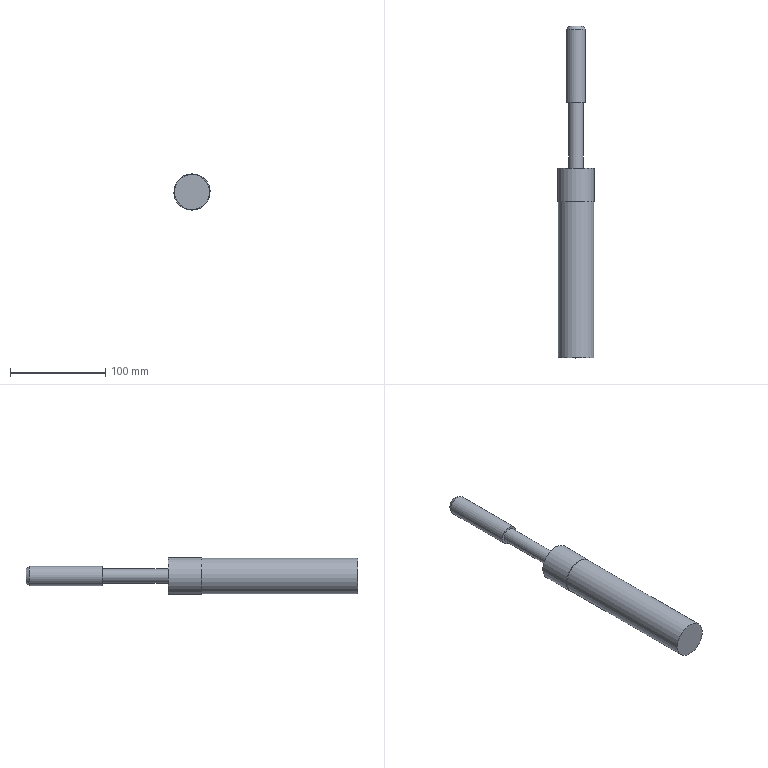Part | STEP file | TOCHA_DE_SOLDA_TBI | 1 solid | 10 faces | box 38 x 348 x 38 mm | volume 253151 mm3 | plane 5 | cylinder 4 | cone 1 | commonest cylinder face diameters 15 x1 20 x1 37 x1 38 x1
STEP:
#1=CARTESIAN_POINT('',(0.,0.,0.));
#2=DIRECTION('',(0.,0.,1.));
#3=DIRECTION('',(1.,0.,0.));
#4=AXIS2_PLACEMENT_3D('',#1,#2,#3);
#5=CARTESIAN_POINT('',(-3.596,-90.,-6.582));
#6=VERTEX_POINT('',#5);
#7=CARTESIAN_POINT('',(0.,-90.,0.));
#8=DIRECTION('',(0.,1.,0.));
#9=DIRECTION('',(1.,0.,0.));
#10=AXIS2_PLACEMENT_3D('',#7,#8,#9);
#11=CIRCLE('',#10,7.5);
#12=CARTESIAN_POINT('',(0.,-184.,0.));
#13=DIRECTION('',(0.,1.,0.));
#14=DIRECTION('',(0.4794,0.,0.8776));
#15=AXIS2_PLACEMENT_3D('',#12,#13,#14);
#16=CYLINDRICAL_SURFACE('',#15,7.5);
#17=CARTESIAN_POINT('',(1.071,94.));
#18=DIRECTION('',(1.,0.));
#19=VECTOR('',#18,1.);
#20=LINE('',#17,#19);
#21=(GEOMETRIC_REPRESENTATION_CONTEXT(2)PARAMETRIC_REPRESENTATION_CONTEXT()REPRESENTATION_CONTEXT('',''));
#22=DEFINITIONAL_REPRESENTATION('',(#20),#21);
#23=PCURVE('',#16,#22);
#24=CARTESIAN_POINT('',(0.,-90.,10.));
#25=DIRECTION('',(0.,1.,0.));
#26=DIRECTION('',(0.,0.,1.));
#27=AXIS2_PLACEMENT_3D('',#24,#25,#26);
#28=PLANE('',#27);
#29=CARTESIAN_POINT('',(-10.,0.));
#30=DIRECTION('',(0.,1.));
#31=AXIS2_PLACEMENT_2D('',#29,#30);
#32=CIRCLE('',#31,7.5);
#33=(GEOMETRIC_REPRESENTATION_CONTEXT(2)PARAMETRIC_REPRESENTATION_CONTEXT()REPRESENTATION_CONTEXT('',''));
#34=DEFINITIONAL_REPRESENTATION('',(#32),#33);
#35=PCURVE('',#28,#34);
#36=SURFACE_CURVE('',#11,(#23,#35),.PCURVE_S1.);
#37=EDGE_CURVE('',#6,#6,#36,.T.);
#38=ORIENTED_EDGE('',*,*,#37,.F.);
#39=CARTESIAN_POINT('',(-3.596,-159.,-6.582));
#40=VERTEX_POINT('',#39);
#41=CARTESIAN_POINT('',(-3.596,-159.,-6.582));
#42=CARTESIAN_POINT('',(-3.596,-90.,-6.582));
#43=B_SPLINE_CURVE_WITH_KNOTS('',1,(#41,#42),.UNSPECIFIED.,.F.,.F.,(2,2),(25.,94.),.PIECEWISE_BEZIER_KNOTS.);
#44=CARTESIAN_POINT('',(3.142,0.));
#45=DIRECTION('',(0.,1.));
#46=VECTOR('',#45,1.);
#47=LINE('',#44,#46);
#48=(GEOMETRIC_REPRESENTATION_CONTEXT(2)PARAMETRIC_REPRESENTATION_CONTEXT()REPRESENTATION_CONTEXT('',''));
#49=DEFINITIONAL_REPRESENTATION('',(#47),#48);
#50=PCURVE('',#16,#49);
#51=CARTESIAN_POINT('',(9.425,0.));
#52=DIRECTION('',(0.,1.));
#53=VECTOR('',#52,1.);
#54=LINE('',#51,#53);
#55=(GEOMETRIC_REPRESENTATION_CONTEXT(2)PARAMETRIC_REPRESENTATION_CONTEXT()REPRESENTATION_CONTEXT('',''));
#56=DEFINITIONAL_REPRESENTATION('',(#54),#55);
#57=PCURVE('',#16,#56);
#58=SEAM_CURVE('',#43,(#50,#57),.PCURVE_S1.);
#59=EDGE_CURVE('',#40,#6,#58,.T.);
#60=ORIENTED_EDGE('',*,*,#59,.F.);
#61=CARTESIAN_POINT('',(0.,-159.,0.));
#62=DIRECTION('',(0.,1.,0.));
#63=DIRECTION('',(1.,0.,0.));
#64=AXIS2_PLACEMENT_3D('',#61,#62,#63);
#65=CIRCLE('',#64,7.5);
#66=CARTESIAN_POINT('',(1.071,25.));
#67=DIRECTION('',(1.,0.));
#68=VECTOR('',#67,1.);
#69=LINE('',#66,#68);
#70=(GEOMETRIC_REPRESENTATION_CONTEXT(2)PARAMETRIC_REPRESENTATION_CONTEXT()REPRESENTATION_CONTEXT('',''));
#71=DEFINITIONAL_REPRESENTATION('',(#69),#70);
#72=PCURVE('',#16,#71);
#73=CARTESIAN_POINT('',(0.,-159.,7.5));
#74=DIRECTION('',(0.,1.,0.));
#75=DIRECTION('',(0.,0.,1.));
#76=AXIS2_PLACEMENT_3D('',#73,#74,#75);
#77=PLANE('',#76);
#78=CARTESIAN_POINT('',(-7.5,0.));
#79=DIRECTION('',(0.,1.));
#80=AXIS2_PLACEMENT_2D('',#78,#79);
#81=CIRCLE('',#80,7.5);
#82=(GEOMETRIC_REPRESENTATION_CONTEXT(2)PARAMETRIC_REPRESENTATION_CONTEXT()REPRESENTATION_CONTEXT('',''));
#83=DEFINITIONAL_REPRESENTATION('',(#81),#82);
#84=PCURVE('',#77,#83);
#85=SURFACE_CURVE('',#65,(#72,#84),.PCURVE_S1.);
#86=EDGE_CURVE('',#40,#40,#85,.T.);
#87=ORIENTED_EDGE('',*,*,#86,.T.);
#88=ORIENTED_EDGE('',*,*,#59,.T.);
#89=EDGE_LOOP('',(#38,#60,#87,#88));
#90=FACE_BOUND('',#89,.T.);
#91=ADVANCED_FACE('',(#90),#16,.T.);
#92=CARTESIAN_POINT('',(-9.109,-159.,-16.674));
#93=VERTEX_POINT('',#92);
#94=CARTESIAN_POINT('',(0.,-159.,0.));
#95=DIRECTION('',(0.,1.,0.));
#96=DIRECTION('',(1.,0.,0.));
#97=AXIS2_PLACEMENT_3D('',#94,#95,#96);
#98=CIRCLE('',#97,19.);
#99=CARTESIAN_POINT('',(0.,-184.,0.));
#100=DIRECTION('',(0.,1.,0.));
#101=DIRECTION('',(0.4794,0.,0.8776));
#102=AXIS2_PLACEMENT_3D('',#99,#100,#101);
#103=CYLINDRICAL_SURFACE('',#102,19.);
#104=CARTESIAN_POINT('',(1.071,25.));
#105=DIRECTION('',(1.,0.));
#106=VECTOR('',#105,1.);
#107=LINE('',#104,#106);
#108=(GEOMETRIC_REPRESENTATION_CONTEXT(2)PARAMETRIC_REPRESENTATION_CONTEXT()REPRESENTATION_CONTEXT('',''));
#109=DEFINITIONAL_REPRESENTATION('',(#107),#108);
#110=PCURVE('',#103,#109);
#111=CARTESIAN_POINT('',(-7.5,0.));
#112=DIRECTION('',(0.,1.));
#113=AXIS2_PLACEMENT_2D('',#111,#112);
#114=CIRCLE('',#113,19.);
#115=(GEOMETRIC_REPRESENTATION_CONTEXT(2)PARAMETRIC_REPRESENTATION_CONTEXT()REPRESENTATION_CONTEXT('',''));
#116=DEFINITIONAL_REPRESENTATION('',(#114),#115);
#117=PCURVE('',#77,#116);
#118=SURFACE_CURVE('',#98,(#110,#117),.PCURVE_S1.);
#119=EDGE_CURVE('',#93,#93,#118,.T.);
#120=ORIENTED_EDGE('',*,*,#119,.F.);
#121=CARTESIAN_POINT('',(-9.109,-194.,-16.674));
#122=VERTEX_POINT('',#121);
#123=CARTESIAN_POINT('',(-9.109,-194.,-16.674));
#124=CARTESIAN_POINT('',(-9.109,-159.,-16.674));
#125=B_SPLINE_CURVE_WITH_KNOTS('',1,(#123,#124),.UNSPECIFIED.,.F.,.F.,(2,2),(-10.,25.),.PIECEWISE_BEZIER_KNOTS.);
#126=CARTESIAN_POINT('',(3.142,0.));
#127=DIRECTION('',(0.,1.));
#128=VECTOR('',#127,1.);
#129=LINE('',#126,#128);
#130=(GEOMETRIC_REPRESENTATION_CONTEXT(2)PARAMETRIC_REPRESENTATION_CONTEXT()REPRESENTATION_CONTEXT('',''));
#131=DEFINITIONAL_REPRESENTATION('',(#129),#130);
#132=PCURVE('',#103,#131);
#133=CARTESIAN_POINT('',(9.425,0.));
#134=DIRECTION('',(0.,1.));
#135=VECTOR('',#134,1.);
#136=LINE('',#133,#135);
#137=(GEOMETRIC_REPRESENTATION_CONTEXT(2)PARAMETRIC_REPRESENTATION_CONTEXT()REPRESENTATION_CONTEXT('',''));
#138=DEFINITIONAL_REPRESENTATION('',(#136),#137);
#139=PCURVE('',#103,#138);
#140=SEAM_CURVE('',#125,(#132,#139),.PCURVE_S1.);
#141=EDGE_CURVE('',#122,#93,#140,.T.);
#142=ORIENTED_EDGE('',*,*,#141,.F.);
#143=CARTESIAN_POINT('',(0.,-194.,0.));
#144=DIRECTION('',(0.,1.,0.));
#145=DIRECTION('',(1.,0.,0.));
#146=AXIS2_PLACEMENT_3D('',#143,#144,#145);
#147=CIRCLE('',#146,19.);
#148=CARTESIAN_POINT('',(1.071,-10.));
#149=DIRECTION('',(1.,0.));
#150=VECTOR('',#149,1.);
#151=LINE('',#148,#150);
#152=(GEOMETRIC_REPRESENTATION_CONTEXT(2)PARAMETRIC_REPRESENTATION_CONTEXT()REPRESENTATION_CONTEXT('',''));
#153=DEFINITIONAL_REPRESENTATION('',(#151),#152);
#154=PCURVE('',#103,#153);
#155=CARTESIAN_POINT('',(0.,-194.,19.));
#156=DIRECTION('',(0.,1.,0.));
#157=DIRECTION('',(0.,0.,1.));
#158=AXIS2_PLACEMENT_3D('',#155,#156,#157);
#159=PLANE('',#158);
#160=CARTESIAN_POINT('',(-19.,0.));
#161=DIRECTION('',(0.,1.));
#162=AXIS2_PLACEMENT_2D('',#160,#161);
#163=CIRCLE('',#162,19.);
#164=(GEOMETRIC_REPRESENTATION_CONTEXT(2)PARAMETRIC_REPRESENTATION_CONTEXT()REPRESENTATION_CONTEXT('',''));
#165=DEFINITIONAL_REPRESENTATION('',(#163),#164);
#166=PCURVE('',#159,#165);
#167=SURFACE_CURVE('',#147,(#154,#166),.PCURVE_S1.);
#168=EDGE_CURVE('',#122,#122,#167,.T.);
#169=ORIENTED_EDGE('',*,*,#168,.T.);
#170=ORIENTED_EDGE('',*,*,#141,.T.);
#171=EDGE_LOOP('',(#120,#142,#169,#170));
#172=FACE_BOUND('',#171,.T.);
#173=ADVANCED_FACE('',(#172),#103,.T.);
#174=CARTESIAN_POINT('',(-8.869,-194.,-16.235));
#175=VERTEX_POINT('',#174);
#176=CARTESIAN_POINT('',(0.,-194.,0.));
#177=DIRECTION('',(0.,1.,0.));
#178=DIRECTION('',(1.,0.,0.));
#179=AXIS2_PLACEMENT_3D('',#176,#177,#178);
#180=CIRCLE('',#179,18.5);
#181=CARTESIAN_POINT('',(0.,-184.,0.));
#182=DIRECTION('',(0.,1.,0.));
#183=DIRECTION('',(0.4794,0.,0.8776));
#184=AXIS2_PLACEMENT_3D('',#181,#182,#183);
#185=CYLINDRICAL_SURFACE('',#184,18.5);
#186=CARTESIAN_POINT('',(1.071,-10.));
#187=DIRECTION('',(1.,0.));
#188=VECTOR('',#187,1.);
#189=LINE('',#186,#188);
#190=(GEOMETRIC_REPRESENTATION_CONTEXT(2)PARAMETRIC_REPRESENTATION_CONTEXT()REPRESENTATION_CONTEXT('',''));
#191=DEFINITIONAL_REPRESENTATION('',(#189),#190);
#192=PCURVE('',#185,#191);
#193=CARTESIAN_POINT('',(-19.,0.));
#194=DIRECTION('',(0.,1.));
#195=AXIS2_PLACEMENT_2D('',#193,#194);
#196=CIRCLE('',#195,18.5);
#197=(GEOMETRIC_REPRESENTATION_CONTEXT(2)PARAMETRIC_REPRESENTATION_CONTEXT()REPRESENTATION_CONTEXT('',''));
#198=DEFINITIONAL_REPRESENTATION('',(#196),#197);
#199=PCURVE('',#159,#198);
#200=SURFACE_CURVE('',#180,(#192,#199),.PCURVE_S1.);
#201=EDGE_CURVE('',#175,#175,#200,.T.);
#202=ORIENTED_EDGE('',*,*,#201,.F.);
#203=CARTESIAN_POINT('',(-8.869,-358.,-16.235));
#204=VERTEX_POINT('',#203);
#205=CARTESIAN_POINT('',(-8.869,-358.,-16.235));
#206=CARTESIAN_POINT('',(-8.869,-194.,-16.235));
#207=B_SPLINE_CURVE_WITH_KNOTS('',1,(#205,#206),.UNSPECIFIED.,.F.,.F.,(2,2),(-174.,-10.),.PIECEWISE_BEZIER_KNOTS.);
#208=CARTESIAN_POINT('',(3.142,0.));
#209=DIRECTION('',(0.,1.));
#210=VECTOR('',#209,1.);
#211=LINE('',#208,#210);
#212=(GEOMETRIC_REPRESENTATION_CONTEXT(2)PARAMETRIC_REPRESENTATION_CONTEXT()REPRESENTATION_CONTEXT('',''));
#213=DEFINITIONAL_REPRESENTATION('',(#211),#212);
#214=PCURVE('',#185,#213);
#215=CARTESIAN_POINT('',(9.425,0.));
#216=DIRECTION('',(0.,1.));
#217=VECTOR('',#216,1.);
#218=LINE('',#215,#217);
#219=(GEOMETRIC_REPRESENTATION_CONTEXT(2)PARAMETRIC_REPRESENTATION_CONTEXT()REPRESENTATION_CONTEXT('',''));
#220=DEFINITIONAL_REPRESENTATION('',(#218),#219);
#221=PCURVE('',#185,#220);
#222=SEAM_CURVE('',#207,(#214,#221),.PCURVE_S1.);
#223=EDGE_CURVE('',#204,#175,#222,.T.);
#224=ORIENTED_EDGE('',*,*,#223,.F.);
#225=CARTESIAN_POINT('',(0.,-358.,0.));
#226=DIRECTION('',(0.,1.,0.));
#227=DIRECTION('',(1.,0.,0.));
#228=AXIS2_PLACEMENT_3D('',#225,#226,#227);
#229=CIRCLE('',#228,18.5);
#230=CARTESIAN_POINT('',(1.071,-174.));
#231=DIRECTION('',(1.,0.));
#232=VECTOR('',#231,1.);
#233=LINE('',#230,#232);
#234=(GEOMETRIC_REPRESENTATION_CONTEXT(2)PARAMETRIC_REPRESENTATION_CONTEXT()REPRESENTATION_CONTEXT('',''));
#235=DEFINITIONAL_REPRESENTATION('',(#233),#234);
#236=PCURVE('',#185,#235);
#237=CARTESIAN_POINT('',(0.,-358.,18.5));
#238=DIRECTION('',(0.,1.,0.));
#239=DIRECTION('',(0.,0.,1.));
#240=AXIS2_PLACEMENT_3D('',#237,#238,#239);
#241=PLANE('',#240);
#242=CARTESIAN_POINT('',(-18.5,0.));
#243=DIRECTION('',(0.,1.));
#244=AXIS2_PLACEMENT_2D('',#242,#243);
#245=CIRCLE('',#244,18.5);
#246=(GEOMETRIC_REPRESENTATION_CONTEXT(2)PARAMETRIC_REPRESENTATION_CONTEXT()REPRESENTATION_CONTEXT('',''));
#247=DEFINITIONAL_REPRESENTATION('',(#245),#246);
#248=PCURVE('',#241,#247);
#249=SURFACE_CURVE('',#229,(#236,#248),.PCURVE_S1.);
#250=EDGE_CURVE('',#204,#204,#249,.T.);
#251=ORIENTED_EDGE('',*,*,#250,.T.);
#252=ORIENTED_EDGE('',*,*,#223,.T.);
#253=EDGE_LOOP('',(#202,#224,#251,#252));
#254=FACE_BOUND('',#253,.T.);
#255=ADVANCED_FACE('',(#254),#185,.T.);
#256=CARTESIAN_POINT('',(-4.794,-90.,-8.776));
#257=VERTEX_POINT('',#256);
#258=CARTESIAN_POINT('',(0.,-90.,0.));
#259=DIRECTION('',(0.,1.,0.));
#260=DIRECTION('',(1.,0.,0.));
#261=AXIS2_PLACEMENT_3D('',#258,#259,#260);
#262=CIRCLE('',#261,10.);
#263=CARTESIAN_POINT('',(-10.,0.));
#264=DIRECTION('',(0.,1.));
#265=AXIS2_PLACEMENT_2D('',#263,#264);
#266=CIRCLE('',#265,10.);
#267=(GEOMETRIC_REPRESENTATION_CONTEXT(2)PARAMETRIC_REPRESENTATION_CONTEXT()REPRESENTATION_CONTEXT('',''));
#268=DEFINITIONAL_REPRESENTATION('',(#266),#267);
#269=PCURVE('',#28,#268);
#270=CARTESIAN_POINT('',(0.,-184.,0.));
#271=DIRECTION('',(0.,1.,0.));
#272=DIRECTION('',(0.4794,0.,0.8776));
#273=AXIS2_PLACEMENT_3D('',#270,#271,#272);
#274=CYLINDRICAL_SURFACE('',#273,10.);
#275=CARTESIAN_POINT('',(1.071,94.));
#276=DIRECTION('',(1.,0.));
#277=VECTOR('',#276,1.);
#278=LINE('',#275,#277);
#279=(GEOMETRIC_REPRESENTATION_CONTEXT(2)PARAMETRIC_REPRESENTATION_CONTEXT()REPRESENTATION_CONTEXT('',''));
#280=DEFINITIONAL_REPRESENTATION('',(#278),#279);
#281=PCURVE('',#274,#280);
#282=SURFACE_CURVE('',#262,(#269,#281),.PCURVE_S1.);
#283=EDGE_CURVE('',#257,#257,#282,.T.);
#284=ORIENTED_EDGE('',*,*,#283,.F.);
#285=EDGE_LOOP('',(#284));
#286=FACE_BOUND('',#285,.T.);
#287=ORIENTED_EDGE('',*,*,#37,.T.);
#288=EDGE_LOOP('',(#287));
#289=FACE_BOUND('',#288,.T.);
#290=ADVANCED_FACE('',(#286,#289),#28,.F.);
#291=ORIENTED_EDGE('',*,*,#119,.T.);
#292=EDGE_LOOP('',(#291));
#293=FACE_BOUND('',#292,.T.);
#294=ORIENTED_EDGE('',*,*,#86,.F.);
#295=EDGE_LOOP('',(#294));
#296=FACE_BOUND('',#295,.T.);
#297=ADVANCED_FACE('',(#293,#296),#77,.T.);
#298=ORIENTED_EDGE('',*,*,#168,.F.);
#299=EDGE_LOOP('',(#298));
#300=FACE_BOUND('',#299,.T.);
#301=ORIENTED_EDGE('',*,*,#201,.T.);
#302=EDGE_LOOP('',(#301));
#303=FACE_BOUND('',#302,.T.);
#304=ADVANCED_FACE('',(#300,#303),#159,.F.);
#305=ORIENTED_EDGE('',*,*,#250,.F.);
#306=EDGE_LOOP('',(#305));
#307=FACE_BOUND('',#306,.T.);
#308=ADVANCED_FACE('',(#307),#241,.F.);
#309=CARTESIAN_POINT('',(-4.794,-13.464,-8.776));
#310=VERTEX_POINT('',#309);
#311=CARTESIAN_POINT('',(0.,-13.464,0.));
#312=DIRECTION('',(0.,1.,0.));
#313=DIRECTION('',(1.,0.,0.));
#314=AXIS2_PLACEMENT_3D('',#311,#312,#313);
#315=CIRCLE('',#314,10.);
#316=CARTESIAN_POINT('',(1.071,170.536));
#317=DIRECTION('',(1.,0.));
#318=VECTOR('',#317,1.);
#319=LINE('',#316,#318);
#320=(GEOMETRIC_REPRESENTATION_CONTEXT(2)PARAMETRIC_REPRESENTATION_CONTEXT()REPRESENTATION_CONTEXT('',''));
#321=DEFINITIONAL_REPRESENTATION('',(#319),#320);
#322=PCURVE('',#274,#321);
#323=CARTESIAN_POINT('',(0.,2.124,0.));
#324=DIRECTION('',(0.,-1.,0.));
#325=DIRECTION('',(-0.4164,0.,-0.9092));
#326=AXIS2_PLACEMENT_3D('',#323,#324,#325);
#327=CONICAL_SURFACE('',#326,1.,0.5236);
#328=CARTESIAN_POINT('',(14.567,15.588));
#329=DIRECTION('',(-1.,0.));
#330=VECTOR('',#329,1.);
#331=LINE('',#328,#330);
#332=(GEOMETRIC_REPRESENTATION_CONTEXT(2)PARAMETRIC_REPRESENTATION_CONTEXT()REPRESENTATION_CONTEXT('',''));
#333=DEFINITIONAL_REPRESENTATION('',(#331),#332);
#334=PCURVE('',#327,#333);
#335=SURFACE_CURVE('',#315,(#322,#334),.PCURVE_S1.);
#336=EDGE_CURVE('',#310,#310,#335,.T.);
#337=ORIENTED_EDGE('',*,*,#336,.F.);
#338=CARTESIAN_POINT('',(-4.794,-90.,-8.776));
#339=CARTESIAN_POINT('',(-4.794,-13.464,-8.776));
#340=B_SPLINE_CURVE_WITH_KNOTS('',1,(#338,#339),.UNSPECIFIED.,.F.,.F.,(2,2),(94.,170.536),.PIECEWISE_BEZIER_KNOTS.);
#341=CARTESIAN_POINT('',(3.142,0.));
#342=DIRECTION('',(0.,1.));
#343=VECTOR('',#342,1.);
#344=LINE('',#341,#343);
#345=(GEOMETRIC_REPRESENTATION_CONTEXT(2)PARAMETRIC_REPRESENTATION_CONTEXT()REPRESENTATION_CONTEXT('',''));
#346=DEFINITIONAL_REPRESENTATION('',(#344),#345);
#347=PCURVE('',#274,#346);
#348=CARTESIAN_POINT('',(9.425,0.));
#349=DIRECTION('',(0.,1.));
#350=VECTOR('',#349,1.);
#351=LINE('',#348,#350);
#352=(GEOMETRIC_REPRESENTATION_CONTEXT(2)PARAMETRIC_REPRESENTATION_CONTEXT()REPRESENTATION_CONTEXT('',''));
#353=DEFINITIONAL_REPRESENTATION('',(#351),#352);
#354=PCURVE('',#274,#353);
#355=SEAM_CURVE('',#340,(#347,#354),.PCURVE_S1.);
#356=EDGE_CURVE('',#257,#310,#355,.T.);
#357=ORIENTED_EDGE('',*,*,#356,.F.);
#358=ORIENTED_EDGE('',*,*,#283,.T.);
#359=ORIENTED_EDGE('',*,*,#356,.T.);
#360=EDGE_LOOP('',(#337,#357,#358,#359));
#361=FACE_BOUND('',#360,.T.);
#362=ADVANCED_FACE('',(#361),#274,.T.);
#363=CARTESIAN_POINT('',(3.835,-10.,7.021));
#364=VERTEX_POINT('',#363);
#365=CARTESIAN_POINT('',(-3.835,-10.,-7.021));
#366=VERTEX_POINT('',#365);
#367=CARTESIAN_POINT('',(0.,-10.,0.));
#368=DIRECTION('',(0.,1.,0.));
#369=DIRECTION('',(1.,0.,0.));
#370=AXIS2_PLACEMENT_3D('',#367,#368,#369);
#371=CIRCLE('',#370,8.);
#372=CARTESIAN_POINT('',(0.,-10.,0.));
#373=DIRECTION('',(0.,1.,0.));
#374=DIRECTION('',(0.,0.,1.));
#375=AXIS2_PLACEMENT_3D('',#372,#373,#374);
#376=PLANE('',#375);
#377=CARTESIAN_POINT('',(0.,0.));
#378=DIRECTION('',(0.,1.));
#379=AXIS2_PLACEMENT_2D('',#377,#378);
#380=CIRCLE('',#379,8.);
#381=(GEOMETRIC_REPRESENTATION_CONTEXT(2)PARAMETRIC_REPRESENTATION_CONTEXT()REPRESENTATION_CONTEXT('',''));
#382=DEFINITIONAL_REPRESENTATION('',(#380),#381);
#383=PCURVE('',#376,#382);
#384=CARTESIAN_POINT('',(14.567,12.124));
#385=DIRECTION('',(-1.,0.));
#386=VECTOR('',#385,1.);
#387=LINE('',#384,#386);
#388=(GEOMETRIC_REPRESENTATION_CONTEXT(2)PARAMETRIC_REPRESENTATION_CONTEXT()REPRESENTATION_CONTEXT('',''));
#389=DEFINITIONAL_REPRESENTATION('',(#387),#388);
#390=PCURVE('',#327,#389);
#391=SURFACE_CURVE('',#371,(#383,#390),.PCURVE_S1.);
#392=EDGE_CURVE('',#364,#366,#391,.T.);
#393=ORIENTED_EDGE('',*,*,#392,.T.);
#394=CARTESIAN_POINT('',(0.,-10.,0.));
#395=DIRECTION('',(0.,1.,0.));
#396=DIRECTION('',(1.,0.,0.));
#397=AXIS2_PLACEMENT_3D('',#394,#395,#396);
#398=CIRCLE('',#397,8.);
#399=CARTESIAN_POINT('',(0.,0.));
#400=DIRECTION('',(0.,1.));
#401=AXIS2_PLACEMENT_2D('',#399,#400);
#402=CIRCLE('',#401,8.);
#403=(GEOMETRIC_REPRESENTATION_CONTEXT(2)PARAMETRIC_REPRESENTATION_CONTEXT()REPRESENTATION_CONTEXT('',''));
#404=DEFINITIONAL_REPRESENTATION('',(#402),#403);
#405=PCURVE('',#376,#404);
#406=CARTESIAN_POINT('',(14.567,12.124));
#407=DIRECTION('',(-1.,0.));
#408=VECTOR('',#407,1.);
#409=LINE('',#406,#408);
#410=(GEOMETRIC_REPRESENTATION_CONTEXT(2)PARAMETRIC_REPRESENTATION_CONTEXT()REPRESENTATION_CONTEXT('',''));
#411=DEFINITIONAL_REPRESENTATION('',(#409),#410);
#412=PCURVE('',#327,#411);
#413=SURFACE_CURVE('',#398,(#405,#412),.PCURVE_S1.);
#414=EDGE_CURVE('',#366,#364,#413,.T.);
#415=ORIENTED_EDGE('',*,*,#414,.T.);
#416=EDGE_LOOP('',(#393,#415));
#417=FACE_BOUND('',#416,.T.);
#418=ADVANCED_FACE('',(#417),#376,.T.);
#419=ORIENTED_EDGE('',*,*,#414,.F.);
#420=CARTESIAN_POINT('',(-3.835,-10.,-7.021));
#421=CARTESIAN_POINT('',(-4.794,-13.464,-8.776));
#422=B_SPLINE_CURVE_WITH_KNOTS('',1,(#420,#421),.UNSPECIFIED.,.F.,.F.,(2,2),(14.,18.),.PIECEWISE_BEZIER_KNOTS.);
#423=CARTESIAN_POINT('',(12.496,0.));
#424=DIRECTION('',(0.,1.));
#425=VECTOR('',#424,1.);
#426=LINE('',#423,#425);
#427=(GEOMETRIC_REPRESENTATION_CONTEXT(2)PARAMETRIC_REPRESENTATION_CONTEXT()REPRESENTATION_CONTEXT('',''));
#428=DEFINITIONAL_REPRESENTATION('',(#426),#427);
#429=PCURVE('',#327,#428);
#430=CARTESIAN_POINT('',(6.213,0.));
#431=DIRECTION('',(0.,1.));
#432=VECTOR('',#431,1.);
#433=LINE('',#430,#432);
#434=(GEOMETRIC_REPRESENTATION_CONTEXT(2)PARAMETRIC_REPRESENTATION_CONTEXT()REPRESENTATION_CONTEXT('',''));
#435=DEFINITIONAL_REPRESENTATION('',(#433),#434);
#436=PCURVE('',#327,#435);
#437=SEAM_CURVE('',#422,(#429,#436),.PCURVE_S1.);
#438=EDGE_CURVE('',#366,#310,#437,.T.);
#439=ORIENTED_EDGE('',*,*,#438,.T.);
#440=ORIENTED_EDGE('',*,*,#336,.T.);
#441=ORIENTED_EDGE('',*,*,#438,.F.);
#442=ORIENTED_EDGE('',*,*,#392,.F.);
#443=EDGE_LOOP('',(#419,#439,#440,#441,#442));
#444=FACE_BOUND('',#443,.T.);
#445=ADVANCED_FACE('',(#444),#327,.T.);
#446=CLOSED_SHELL('',(#91,#173,#255,#290,#297,#304,#308,#362,#418,#445));
#447=MANIFOLD_SOLID_BREP('',#446);
#448=(LENGTH_UNIT()NAMED_UNIT(*)SI_UNIT(.MILLI.,.METRE.));
#449=UNCERTAINTY_MEASURE_WITH_UNIT(LENGTH_MEASURE(0.000005),#448,'','');
#450=(NAMED_UNIT(*)PLANE_ANGLE_UNIT()SI_UNIT($,.RADIAN.));
#451=(NAMED_UNIT(*)SI_UNIT($,.STERADIAN.)SOLID_ANGLE_UNIT());
#452=(GEOMETRIC_REPRESENTATION_CONTEXT(3)GLOBAL_UNCERTAINTY_ASSIGNED_CONTEXT((#449))GLOBAL_UNIT_ASSIGNED_CONTEXT((#448,#450,#451))REPRESENTATION_CONTEXT('',''));
#453=ADVANCED_BREP_SHAPE_REPRESENTATION('',(#4,#447),#452);